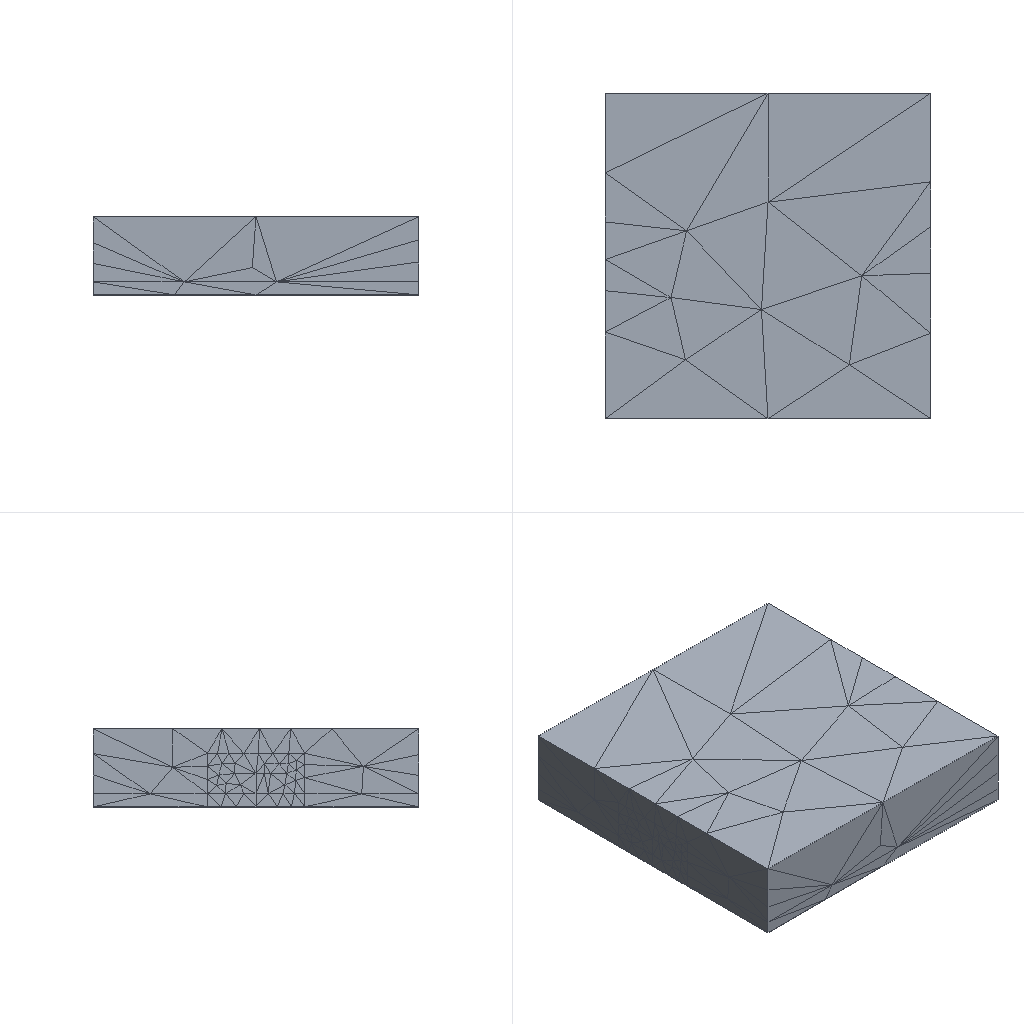Simulation study | ansys electronics desktop
Set-up summary:
category,name,step,type,value,unit,region
solver,ansys_electronics_desktop
units,length mm,,stated,model units
analysis,M15,,HFSS Modal Network,design_type=HFSS
setup,Setup1,M15,HfssDriven,frequency=2.5GHz; max_passes=2; max_delta_s=0.08
sweep,Sweep1,Setup1,Interpolating,1GHz..5GHz n=11 step=
mesh,nodes,,,n/a (no mesh stored)
mesh,elements,,,n/a (no mesh stored)
material,vacuum,,permittivity,1
load,P1,M15,wave port,,,objects 132
load,P2,M15,wave port,,,objects 144
bc,PerfE_TWX736,M15,perfect e,,,objects 118
Ansys Electronics Desktop project file, long lists of numbers shortened, first 729 of 3453 lines:
$begin 'AnsoftProject'
	Created='Wed Sep 30 18:16:02 2026'
	Product='ElectronicsDesktop'
	FileOwnedByWorkbench=false
	$begin 'Desktop'
		Version(2026, 1)
		InfrastructureVersion(1, 0)
		$begin 'FactoryHeader'
			$begin 'geometry3deditor'
				KernelVersion(2, 0)
				ProjectContainsGeometry3D='1'
			$end 'geometry3deditor'
		$end 'FactoryHeader'
	$end 'Desktop'
	UsesAdvancedFeatures=false
	PreviewImageDesignId=1
	NextUniqueID=0
	MoveBackwards=false
	$begin 'HFSSEnvironment'
		Version(1, 0)
	$end 'HFSSEnvironment'
	$begin 'PlanarEMEnvironment'
		Version(1, 0)
	$end 'PlanarEMEnvironment'
	$begin 'Q3DEnvironment'
		Version(1, 0)
	$end 'Q3DEnvironment'
	$begin '2DExtractorEnvironment'
		Version(1, 0)
	$end '2DExtractorEnvironment'
	$begin 'NexximEnvironment'
		Version(1, 0)
	$end 'NexximEnvironment'
	$begin 'NexximNetlistEnvironment'
		Version(1, 0)
	$end 'NexximNetlistEnvironment'
	$begin 'EmitEnvironment'
		Version(1, 0)
	$end 'EmitEnvironment'
	$begin 'Maxwell3DEnvironment'
		Version(1, 0)
	$end 'Maxwell3DEnvironment'
	$begin 'Maxwell2DEnvironment'
		Version(1, 0)
	$end 'Maxwell2DEnvironment'
	$begin 'RMxprtEnvironment'
		Version(1, 0)
	$end 'RMxprtEnvironment'
	$begin 'MaxCirEnvironment'
		Version(1, 0)
	$end 'MaxCirEnvironment'
	$begin 'SimplorerEnvironment'
		Version(1, 0)
	$end 'SimplorerEnvironment'
	$begin 'IcepakEnvironment'
		Version(1, 0)
	$end 'IcepakEnvironment'
	$begin 'IcepakFEAEnvironment'
		Version(1, 0)
	$end 'IcepakFEAEnvironment'
	$begin 'SchematicEnvironment'
		Version(1, 0)
	$end 'SchematicEnvironment'
	$begin 'geometry3deditor'
		Version(1, 0)
	$end 'geometry3deditor'
	ReadVersion=12
	$begin 'DesignMgrEnvironment'
		CompInstCounter=1
		GPortCounter=0
		NetCounter=0
		Alias('Ieee;Simplorer Elements\\Ieee', 'Std;Simplorer Elements\\Std', 'Basic_VHDLAMS;Simplorer Elements\\Basic Elements VHDLAMS\\Basic Elements VHDLAMS', 'Digital_Elements;Simplorer Elements\\Digital Elements\\Digital Elements', 'Transformations;Simplorer Elements\\Tools\\Transformations\\Transformations', 'HEV_VHDLAMS;Simplorer Elements\\HEV VHDLAMS\\HEV VHDLAMS', 'automotive_vda;Simplorer Elem
	$end 'DesignMgrEnvironment'
	$begin 'ProjectDatasets'
		NextUniqueID=0
		MoveBackwards=false
		DatasetType='ProjectDatasetType'
		$begin 'DatasetDefinitions'
		$end 'DatasetDefinitions'
	$end 'ProjectDatasets'
	VariableOrders[0:]
	$begin 'Definitions'
		$begin 'Materials'
			$begin 'vacuum'
				CoordinateSystemType='Cartesian'
				BulkOrSurfaceType=1
				$begin 'PhysicsTypes'
					set('Electromagnetic')
				$end 'PhysicsTypes'
				$begin 'AttachedData'
					$begin 'MatAppearanceData'
						property_data='appearance_data'
						Red=230
						Green=230
						Blue=230
						Transparency=0.95
					$end 'MatAppearanceData'
				$end 'AttachedData'
				permittivity='1'
				ModTime=1499970477
				Library='Materials'
				LibLocation='SysLibrary'
				ModSinceLib=false
			$end 'vacuum'
		$end 'Materials'
		$begin 'SurfaceMaterials'
		$end 'SurfaceMaterials'
		$begin 'Scripts'
		$end 'Scripts'
		$begin 'AnsysComponents'
			NextUniqueID=0
			MoveBackwards=false
			$begin 'AnsysComponentDefinitions'
			$end 'AnsysComponentDefinitions'
		$end 'AnsysComponents'
		$begin 'Symbols'
			$begin 'M15'
				ModTime=1790763363
				Library=''
				ModSinceLib=false
				LibLocation='Project'
				HighestLevel=1
				Normalize=true
				InitialLevels(0, 1)
				$begin 'Graphics'
					Rect(0, 0, 0, 0, 0.00254, 0.00254, 0.00508, 0.00508, 0, 0, 0)
					Rect(0, 1, 0, 0, 0.0004233, 0.00254, 0.0004233, 0.0004233, 0, 0, 0)
				$end 'Graphics'
			$end 'M15'
		$end 'Symbols'
		$begin 'DefInfo'
			M15(1002, 0, 0, 0, '', 1790763363, '', 'M15', '', '', '', '', '', 'Design.bmp', '', 'Project', '', '', 1790763363, '', 0, 0)
		$end 'DefInfo'
		$begin 'Compdefs'
			$begin 'M15'
				Library=''
				CircuitEnv=0
				Refbase='U'
				NumParts=1
				ModSinceLib=true
				$begin 'Properties'
					TextProp('Representation', 'SRD', '', 'M15')
					TextProp('Owner', 'SRD', '', 'HFSS')
				$end 'Properties'
				CompExtID=6
				$begin 'Parameters'
					ButtonProp('CosimDefinition', 'D', '', 'Edit', 'Edit', 40501, ButtonPropClientData())
					MenuProp('CoSimulator', 'D', '', 'DefaultNetlist', 0)
				$end 'Parameters'
				$begin 'CosimDefinitions'
					$begin 'CosimDefinition'
						CosimulatorType=4
						CosimDefName='DefaultNetlist'
						IsDefinition=true
						Connect=true
						Data()
						GRef()
					$end 'CosimDefinition'
					DefaultCosim='DefaultNetlist'
				$end 'CosimDefinitions'
			$end 'M15'
		$end 'Compdefs'
	$end 'Definitions'
	DesignIDServer=2
	MoveBackwards=false
	$begin 'HFSSModel'
		RepRewriteV2=true
		Name='M15'
		DesignID=0
		'Use Advanced DC Extrapolation'=false
		'Use Power S'=false
		'Export FRTM After Simulation'=false
		'Export Rays After Simulation'=false
		'Export After Simulation'=false
		'Allow Material Override'=false
		'Calculate Lossy Dielectrics'=false
		'Perform Minimal validation'=false
		$begin 'TemperatureSettings'
			IncludeTemperatureDependence=false
			EnableFeedback=false
			Temperatures(6, '22cel', 34, '22cel', 62, '22cel', 90, '22cel', 118, '22cel', 132, '22cel', 144, '22cel', 156, '22cel')
		$end 'TemperatureSettings'
		ObjsEnabledForDeformation()
		'Port Validation Settings'='Standard'
		'Save Adaptive support files'=false
		SolutionType='HFSS Modal Network'
		$begin 'DrivenOptions'
			AutoOpen=false
		$end 'DrivenOptions'
		HasTransientSetups=false
		MaterialDensity=1
		MassOfTissue=1
		VoxelSize=1
		TissueObjectList=-1
		AverageSarMethod=0
		UseAutoDCThickness=true
		HaveZwaveSupport=true
		SolveInsideThreshold=100000
		RequireBodyFaceInfo=false
		$begin 'OutputVariable'
			NextUniqueID=0
			MoveBackwards=false
		$end 'OutputVariable'
		$begin 'ModelSetup'
			$begin 'DesignDatasets'
				NextUniqueID=0
				MoveBackwards=false
				DatasetType='DesignDatasetType'
				$begin 'DatasetDefinitions'
				$end 'DatasetDefinitions'
			$end 'DesignDatasets'
			VariableOrders[0:]
			$begin 'Editor3D Doc Preferences'
				BackgroundColorVersion=1
				'Plane Background'=0
				'Need Lights'=true
				'Ambient Light'=8355711
				'Num Lights'=1
				Light0[4: 16777215, 0.75, -0.15, -0.63]
				Ver=2
			$end 'Editor3D Doc Preferences'
			SnapMode=31
			WorkingCS=1
			$begin 'GeometryCore'
				BlockVersionID=3
				DataVersion=2
				NativeKernel='PARASOLID'
				NativeKernelVersionID=26
				Units='mm'
				ModelExtents=10000
				InstanceID=-1
				$begin 'ValidationOptions'
					EntityCheckLevel='Strict'
					IgnoreUnclassifiedObjects=false
					SkipIntersectionChecks=false
				$end 'ValidationOptions'
				ContainsGeomLinkUDM=false
				$begin 'GeometryOperations'
					BlockVersionID=2
					$begin 'AnsoftRangedIDServerManager'
						$begin 'AnsoftRangedIDServer'
							IDServerObjectTypeID=0
							IDServerRangeMin=0
							IDServerRangeMax=2146483647
							NextUniqueID=183
							MoveBackwards=false
						$end 'AnsoftRangedIDServer'
						$begin 'AnsoftRangedIDServer'
							IDServerObjectTypeID=1
							IDServerRangeMin=2146483648
							IDServerRangeMax=2146485547
							NextUniqueID=2146483654
							MoveBackwards=false
						$end 'AnsoftRangedIDServer'
					$end 'AnsoftRangedIDServerManager'
					StartBackGroundFaceID=2146483648
					$begin 'CoordinateSystems'
					$end 'CoordinateSystems'
					$begin 'OperandCSs'
					$end 'OperandCSs'
					$begin 'SubModelDefinitions'
					$end 'SubModelDefinitions'
					$begin 'Groups'
					$end 'Groups'
					$begin 'UserDefinedModels'
					$end 'UserDefinedModels'
					$begin 'OperandUserDefinedModels'
					$end 'OperandUserDefinedModels'
					$begin 'ToplevelParts'
						$begin 'GeometryPart'
							$begin 'Attributes'
								Name='Sub'
								Flags=''
								Color='(230 230 230)'
								Transparency=0.8
								PartCoordinateSystem=1
								UDMId=-1
								GroupId=-1
								MaterialValue='"vacuum"'
								SurfaceMaterialValue='""'
								SolveInside=true
								ShellElement=false
								ShellElementThickness='0mm'
								ReferenceTemperature='20cel'
								IsMaterialEditable=true
								IsSurfaceMaterialEditable=true
								UseMaterialAppearance=false
								IsLightweight=false
								IsAlwaysHidden=false
							$end 'Attributes'
							$begin 'PhysicsAttributes'
								SuppressedForPhysics='False'
								SuppressedForPhysicsEditable=true
							$end 'PhysicsAttributes'
							$begin 'Operations'
								$begin 'Operation'
									OperationType='Box'
									ID=5
									ReferenceCoordSystemID=1
									$begin 'BoxParameters'
										KernelVersion=23
										XPosition='-20mm'
										YPosition='-20mm'
										ZPosition='-1.6mm'
										XSize='40mm'
										YSize='40mm'
										ZSize='1.6mm'
									$end 'BoxParameters'
									ParentPartID=6
									ReferenceUDMID=-1
									IsSuppressed=false
									$begin 'OperationIdentity'
										$begin 'Topology'
											NumLumps=1
											NumShells=1
											NumFaces=6
											NumWires=0
											NumLoops=6
											NumCoedges=24
											NumEdges=12
											NumVertices=8
										$end 'Topology'
										BodyID=6
										StartFaceID=7
										StartEdgeID=13
										StartVertexID=25
										NumNewFaces=6
										NumNewEdges=12
										NumNewVertices=8
										FaceNameAndIDMap()
										EdgeNameAndIDMap()
										VertexNameAndIDMap()
									$end 'OperationIdentity'
								$end 'Operation'
							$end 'Operations'
							$begin 'SubregionDependencyInformation'
								ChildSubregions[0:]
							$end 'SubregionDependencyInformation'
						$end 'GeometryPart'
						$begin 'GeometryPart'
							$begin 'Attributes'
								Name='GND'
								Flags=''
								Color='(230 230 230)'
								Transparency=0.8
								PartCoordinateSystem=1
								UDMId=-1
								GroupId=-1
								MaterialValue='"vacuum"'
								SurfaceMaterialValue='""'
								SolveInside=true
								ShellElement=false
								ShellElementThickness='0mm'
								ReferenceTemperature='20cel'
								IsMaterialEditable=true
								IsSurfaceMaterialEditable=true
								UseMaterialAppearance=false
								IsLightweight=false
								IsAlwaysHidden=false
							$end 'Attributes'
							$begin 'PhysicsAttributes'
								SuppressedForPhysics='False'
								SuppressedForPhysicsEditable=true
							$end 'PhysicsAttributes'
							$begin 'Operations'
								$begin 'Operation'
									OperationType='Box'
									ID=33
									ReferenceCoordSystemID=1
									$begin 'BoxParameters'
										KernelVersion=23
										XPosition='-20mm'
										YPosition='-20mm'
										ZPosition='-1.635mm'
										XSize='40mm'
										YSize='40mm'
										ZSize='0.035mm'
									$end 'BoxParameters'
									ParentPartID=34
									ReferenceUDMID=-1
									IsSuppressed=false
									$begin 'OperationIdentity'
										$begin 'Topology'
											NumLumps=1
											NumShells=1
											NumFaces=6
											NumWires=0
											NumLoops=6
											NumCoedges=24
											NumEdges=12
											NumVertices=8
										$end 'Topology'
										BodyID=34
										StartFaceID=35
										StartEdgeID=41
										StartVertexID=53
										NumNewFaces=6
										NumNewEdges=12
										NumNewVertices=8
										FaceNameAndIDMap()
										EdgeNameAndIDMap()
										VertexNameAndIDMap()
									$end 'OperationIdentity'
								$end 'Operation'
							$end 'Operations'
							$begin 'SubregionDependencyInformation'
								ChildSubregions[0:]
							$end 'SubregionDependencyInformation'
						$end 'GeometryPart'
						$begin 'GeometryPart'
							$begin 'Attributes'
								Name='F1'
								Flags=''
								Color='(230 230 230)'
								Transparency=0.8
								PartCoordinateSystem=1
								UDMId=-1
								GroupId=-1
								MaterialValue='"vacuum"'
								SurfaceMaterialValue='""'
								SolveInside=true
								ShellElement=false
								ShellElementThickness='0mm'
								ReferenceTemperature='20cel'
								IsMaterialEditable=true
								IsSurfaceMaterialEditable=true
								UseMaterialAppearance=false
								IsLightweight=false
								IsAlwaysHidden=false
							$end 'Attributes'
							$begin 'PhysicsAttributes'
								SuppressedForPhysics='False'
								SuppressedForPhysicsEditable=true
							$end 'PhysicsAttributes'
							$begin 'Operations'
								$begin 'Operation'
									OperationType='Box'
									ID=61
									ReferenceCoordSystemID=1
									$begin 'BoxParameters'
										KernelVersion=23
										XPosition='-20mm'
										YPosition='-1.5mm'
										ZPosition='0mm'
										XSize='12mm'
										YSize='3mm'
										ZSize='0.035mm'
									$end 'BoxParameters'
									ParentPartID=62
									ReferenceUDMID=-1
									IsSuppressed=false
									$begin 'OperationIdentity'
										$begin 'Topology'
											NumLumps=1
											NumShells=1
											NumFaces=6
											NumWires=0
											NumLoops=6
											NumCoedges=24
											NumEdges=12
											NumVertices=8
										$end 'Topology'
										BodyID=62
										StartFaceID=63
										StartEdgeID=69
										StartVertexID=81
										NumNewFaces=6
										NumNewEdges=12
										NumNewVertices=8
										FaceNameAndIDMap()
										EdgeNameAndIDMap()
										VertexNameAndIDMap()
									$end 'OperationIdentity'
								$end 'Operation'
							$end 'Operations'
							$begin 'SubregionDependencyInformation'
								ChildSubregions[0:]
							$end 'SubregionDependencyInformation'
						$end 'GeometryPart'
						$begin 'GeometryPart'
							$begin 'Attributes'
								Name='F2'
								Flags=''
								Color='(230 230 230)'
								Transparency=0.8
								PartCoordinateSystem=1
								UDMId=-1
								GroupId=-1
								MaterialValue='"vacuum"'
								SurfaceMaterialValue='""'
								SolveInside=true
								ShellElement=false
								ShellElementThickness='0mm'
								ReferenceTemperature='20cel'
								IsMaterialEditable=true
								IsSurfaceMaterialEditable=true
								UseMaterialAppearance=false
								IsLightweight=false
								IsAlwaysHidden=false
							$end 'Attributes'
							$begin 'PhysicsAttributes'
								SuppressedForPhysics='False'
								SuppressedForPhysicsEditable=true
							$end 'PhysicsAttributes'
							$begin 'Operations'
								$begin 'Operation'
									OperationType='Box'
									ID=89
									ReferenceCoordSystemID=1
									$begin 'BoxParameters'
										KernelVersion=23
										XPosition='8mm'
										YPosition='-1.5mm'
										ZPosition='0mm'
										XSize='12mm'
										YSize='3mm'
										ZSize='0.035mm'
									$end 'BoxParameters'
									ParentPartID=90
									ReferenceUDMID=-1
									IsSuppressed=false
									$begin 'OperationIdentity'
										$begin 'Topology'
											NumLumps=1
											NumShells=1
											NumFaces=6
											NumWires=0
											NumLoops=6
											NumCoedges=24
											NumEdges=12
											NumVertices=8
										$end 'Topology'
										BodyID=90
										StartFaceID=91
										StartEdgeID=97
										StartVertexID=109
										NumNewFaces=6
										NumNewEdges=12
										NumNewVertices=8
										FaceNameAndIDMap()
										EdgeNameAndIDMap()
										VertexNameAndIDMap()
									$end 'OperationIdentity'
								$end 'Operation'
							$end 'Operations'
							$begin 'SubregionDependencyInformation'
								ChildSubregions[0:]
							$end 'SubregionDependencyInformation'
						$end 'GeometryPart'
						$begin 'GeometryPart'
							$begin 'Attributes'
								Name='RingO'
								Flags=''
								Color='(230 230 230)'
								Transparency=0.8
								PartCoordinateSystem=1
								UDMId=-1
								GroupId=-1
								MaterialValue='"vacuum"'
								SurfaceMaterialValue='""'
								SolveInside=true
								ShellElement=false
								ShellElementThickness='0mm'
								ReferenceTemperature='20cel'
								IsMaterialEditable=true
								IsSurfaceMaterialEditable=true
								UseMaterialAppearance=false
								IsLightweight=false
								IsAlwaysHidden=false
							$end 'Attributes'
							$begin 'PhysicsAttributes'
								SuppressedForPhysics='False'
								SuppressedForPhysicsEditable=true
							$end 'PhysicsAttributes'
							$begin 'Operations'
								$begin 'Operation'
									OperationType='Circle'
									ID=117
									ReferenceCoordSystemID=1
									$begin 'CircleParameters'
										KernelVersion=23
										XCenter='0mm'
										YCenter='0mm'
										ZCenter='0mm'
										Radius='10mm'
										WhichAxis='Z'
										NumSegments='0'
									$end 'CircleParameters'
									ParentPartID=118
									ReferenceUDMID=-1
									IsSuppressed=false
									$begin 'OperationIdentity'
										$begin 'Topology'
											NumLumps=1
											NumShells=1
											NumFaces=0
											NumWires=1
											NumLoops=0
											NumCoedges=0
											NumEdges=1
											NumVertices=0
										$end 'Topology'
										BodyID=118
										StartFaceID=-1
										StartEdgeID=119
										StartVertexID=-1
										NumNewFaces=0
										NumNewEdges=1
										NumNewVertices=0
										FaceNameAndIDMap()
										EdgeNameAndIDMap()
										VertexNameAndIDMap()
									$end 'OperationIdentity'
								$end 'Operation'
								$begin 'Operation'
									OperationType='CoverLines'
									ID=121
									$begin 'LocalOperationParameters'
										KernelVersion=23
										LocalOpPart=118
									$end 'LocalOperationParameters'
									ParentPartID=118
									ReferenceUDMID=-1
									IsSuppressed=false
									$begin 'OperationIdentity'
										$begin 'Topology'
											NumLumps=1
											NumShells=1
											NumFaces=1
											NumWires=0
											NumLoops=1
											NumCoedges=1
											NumEdges=1
											NumVertices=0
										$end 'Topology'
										BodyID=-1
										StartFaceID=122
										StartEdgeID=-1
										StartVertexID=-1
										NumNewFaces=1
										NumNewEdges=0
										NumNewVertices=0
										FaceNameAndIDMap()
										EdgeNameAndIDMap()
										VertexNameAndIDMap()
										$begin 'GeomTopolBasedOperationIdentityHelper'
											$begin 'NewFaces'
												$begin 'Face'
													NormalizedSerialNum=0
													ID=122
													$begin 'FaceGeomTopol'
														FaceTopol(1, 1, 1, 0)
														$begin 'FaceGeometry'
															Area=314.159
															FcUVMid(0, 0, 0)
															$begin 'FcTolVts'
															$end 'FcTolVts'
														$end 'FaceGeometry'
													$end 'FaceGeomTopol'
												$end 'Face'
											$end 'NewFaces'
											$begin 'NewEdges'
											$end 'NewEdges'
											$begin 'NewVertices'
											$end 'NewVertices'
										$end 'GeomTopolBasedOperationIdentityHelper'
									$end 'OperationIdentity'
									ParentOperationID=117
								$end 'Operation'
								$begin 'Operation'
									OperationType='Substract'
									ID=129
									$begin 'SubtractParameters'
										KernelVersion=23
										KeepOriginals=false
										TurnOnNBodyBoolean=false
										BlankPart=118
										NumToolParts=1
										ToolParts(124)
									$end 'SubtractParameters'
									ParentPartID=118
									ReferenceUDMID=-1
									IsSuppressed=false
									$begin 'OperationIdentity'
										$begin 'Topology'
											NumLumps=1
											NumShells=1
											NumFaces=1
											NumWires=0
											NumLoops=2
											NumCoedges=2
											NumEdges=2
											NumVertices=0
										$end 'Topology'
										BodyID=-1
										StartFaceID=-1
										StartEdgeID=130
										StartVertexID=-1
										NumNewFaces=0
										NumNewEdges=1
										NumNewVertices=0
										FaceNameAndIDMap()
										EdgeNameAndIDMap()
										VertexNameAndIDMap()
										$begin 'GeomTopolBasedOperationIdentityHelper'
											$begin 'NewFaces'
											$end 'NewFaces'
											$begin 'NewEdges'
												$begin 'Edge'
													NormalizedSerialNum=0
													ID=130
													EdgeFaces(122)
													$begin 'EdTolVts'
													$end 'EdTolVts'
													EdgeMidPoint(-8, 9.79717439317883e-16, 0)
												$end 'Edge'
											$end 'NewEdges'
											$begin 'NewVertices'
											$end 'NewVertices'
										$end 'GeomTopolBasedOperationIdentityHelper'
										$begin 'MergedFaces'
										$end 'MergedFaces'
										$begin 'MergedEdges'
										$end 'MergedEdges'
									$end 'OperationIdentity'
									BlankOperation=121
									NumToolOperations=1
									ToolOperations(127)
								$end 'Operation'
Last 1318 lines:
														$end 'LegendTableAttrib'
														LegendName=''
														ShowTraceName=true
														ShowSolutionName=true
														ShowVariationKey=true
														FileNameDisplayModeInVariationKey=0
														DockMode='None'
													$end 'LegendRenderAttribute'
												$end 'SubMapItem'
											$end 'MainMapItem'
											$begin 'MainMapItem'
												$begin 'SubMapItem'
													DataSourceID=1
													$begin 'LineAxisRenderAttribute'
														DecimalFieldWidth=3
														DecimalFieldPrecision=2
														ManualTitle=''
														ColorVersion=1
														MinScale=0
														MaxScale=1
														TickSpacing=1
														ManualUnits=false
														Units='mm'
														AxisScale='Linear'
														NumberFormat='Auto'
														$begin 'TextFont'
															$begin 'FontAttribute'
																$begin 'Font'
																	HeightInPts=9
																	Width=0
																	Escapement=0
																	Orientation=0
																	Weight=400
																	Italic=0
																	Underline=0
																	StrikeOut=0
																	CharSet=0
																	OutPrecision=7
																	ClipPrecision=48
																	Quality=6
																	PitchAndFamily=0
																	FaceName='Arial'
																$end 'Font'
																ColorVersion=1
															$end 'FontAttribute'
														$end 'TextFont'
														InfMapMode=false
														InfMapValue=1.79769313486232e+306
														AutoRangeMin=true
														AutoRangeMax=true
														AutoSpacing=true
														kNumMinorDivisions=5
														ShowAxisTitle=true
														ShowAxisUnits=true
														vwm='FullWnd'
														viewWndWd=#nan
														ActivateMargins=true
														MarginPercent=0
														NeverCollapse=false
														AxisStripes=true
													$end 'LineAxisRenderAttribute'
												$end 'SubMapItem'
												$begin 'SubMapItem'
													DataSourceID=2
													$begin 'LineAxisRenderAttribute'
														DecimalFieldWidth=3
														DecimalFieldPrecision=2
														ManualTitle=''
														ColorVersion=1
														MinScale=0
														MaxScale=1
														TickSpacing=1
														ManualUnits=false
														Units='mm'
														AxisScale='Linear'
														NumberFormat='Auto'
														$begin 'TextFont'
															$begin 'FontAttribute'
																$begin 'Font'
																	HeightInPts=9
																	Width=0
																	Escapement=0
																	Orientation=0
																	Weight=400
																	Italic=0
																	Underline=0
																	StrikeOut=0
																	CharSet=0
																	OutPrecision=7
																	ClipPrecision=48
																	Quality=6
																	PitchAndFamily=0
																	FaceName='Arial'
																$end 'Font'
																ColorVersion=1
															$end 'FontAttribute'
														$end 'TextFont'
														InfMapMode=false
														InfMapValue=1.79769313486232e+306
														AutoRangeMin=true
														AutoRangeMax=true
														AutoSpacing=true
														kNumMinorDivisions=5
														ShowAxisTitle=true
														ShowAxisUnits=true
														vwm='FullWnd'
														viewWndWd=#nan
														ActivateMargins=true
														MarginPercent=0
														NeverCollapse=false
														AxisStripes=true
													$end 'LineAxisRenderAttribute'
												$end 'SubMapItem'
												$begin 'SubMapItem'
													DataSourceID=8
													$begin 'LineAxisRenderAttribute'
														DecimalFieldWidth=3
														DecimalFieldPrecision=2
														ManualTitle=''
														ColorVersion=1
														MinScale=0
														MaxScale=1
														TickSpacing=1
														ManualUnits=false
														Units='mm'
														AxisScale='Linear'
														NumberFormat='Auto'
														$begin 'TextFont'
															$begin 'FontAttribute'
																$begin 'Font'
																	HeightInPts=9
																	Width=0
																	Escapement=0
																	Orientation=0
																	Weight=400
																	Italic=0
																	Underline=0
																	StrikeOut=0
																	CharSet=0
																	OutPrecision=7
																	ClipPrecision=48
																	Quality=6
																	PitchAndFamily=0
																	FaceName='Arial'
																$end 'Font'
																ColorVersion=1
															$end 'FontAttribute'
														$end 'TextFont'
														InfMapMode=false
														InfMapValue=1.79769313486232e+306
														AutoRangeMin=true
														AutoRangeMax=true
														AutoSpacing=true
														kNumMinorDivisions=5
														ShowAxisTitle=true
														ShowAxisUnits=true
														vwm='FullWnd'
														viewWndWd=#nan
														ActivateMargins=true
														MarginPercent=0
														NeverCollapse=false
														AxisStripes=true
													$end 'LineAxisRenderAttribute'
												$end 'SubMapItem'
												$begin 'SubMapItem'
													DataSourceID=9
													$begin 'LineAxisRenderAttribute'
														DecimalFieldWidth=3
														DecimalFieldPrecision=2
														ManualTitle=''
														ColorVersion=1
														MinScale=0
														MaxScale=1
														TickSpacing=1
														ManualUnits=false
														Units='mm'
														AxisScale='Linear'
														NumberFormat='Auto'
														$begin 'TextFont'
															$begin 'FontAttribute'
																$begin 'Font'
																	HeightInPts=9
																	Width=0
																	Escapement=0
																	Orientation=0
																	Weight=400
																	Italic=0
																	Underline=0
																	StrikeOut=0
																	CharSet=0
																	OutPrecision=7
																	ClipPrecision=48
																	Quality=6
																	PitchAndFamily=0
																	FaceName='Arial'
																$end 'Font'
																ColorVersion=1
															$end 'FontAttribute'
														$end 'TextFont'
														InfMapMode=false
														InfMapValue=1.79769313486232e+306
														AutoRangeMin=true
														AutoRangeMax=true
														AutoSpacing=true
														kNumMinorDivisions=5
														ShowAxisTitle=true
														ShowAxisUnits=true
														vwm='FullWnd'
														viewWndWd=#nan
														ActivateMargins=true
														MarginPercent=0
														NeverCollapse=false
														AxisStripes=true
													$end 'LineAxisRenderAttribute'
												$end 'SubMapItem'
												$begin 'SubMapItem'
													DataSourceID=10
													$begin 'LineAxisRenderAttribute'
														DecimalFieldWidth=3
														DecimalFieldPrecision=2
														ManualTitle=''
														ColorVersion=1
														MinScale=0
														MaxScale=1
														TickSpacing=1
														ManualUnits=false
														Units='mm'
														AxisScale='Linear'
														NumberFormat='Auto'
														$begin 'TextFont'
															$begin 'FontAttribute'
																$begin 'Font'
																	HeightInPts=9
																	Width=0
																	Escapement=0
																	Orientation=0
																	Weight=400
																	Italic=0
																	Underline=0
																	StrikeOut=0
																	CharSet=0
																	OutPrecision=7
																	ClipPrecision=48
																	Quality=6
																	PitchAndFamily=0
																	FaceName='Arial'
																$end 'Font'
																ColorVersion=1
															$end 'FontAttribute'
														$end 'TextFont'
														InfMapMode=false
														InfMapValue=1.79769313486232e+306
														AutoRangeMin=true
														AutoRangeMax=true
														AutoSpacing=true
														kNumMinorDivisions=5
														ShowAxisTitle=true
														ShowAxisUnits=true
														vwm='FullWnd'
														viewWndWd=#nan
														ActivateMargins=true
														MarginPercent=0
														NeverCollapse=false
														AxisStripes=true
													$end 'LineAxisRenderAttribute'
												$end 'SubMapItem'
												$begin 'SubMapItem'
													DataSourceID=11
													$begin 'LineAxisRenderAttribute'
														DecimalFieldWidth=3
														DecimalFieldPrecision=2
														ManualTitle=''
														ColorVersion=1
														MinScale=0
														MaxScale=1
														TickSpacing=1
														ManualUnits=false
														Units='mm'
														AxisScale='Linear'
														NumberFormat='Auto'
														$begin 'TextFont'
															$begin 'FontAttribute'
																$begin 'Font'
																	HeightInPts=9
																	Width=0
																	Escapement=0
																	Orientation=0
																	Weight=400
																	Italic=0
																	Underline=0
																	StrikeOut=0
																	CharSet=0
																	OutPrecision=7
																	ClipPrecision=48
																	Quality=6
																	PitchAndFamily=0
																	FaceName='Arial'
																$end 'Font'
																ColorVersion=1
															$end 'FontAttribute'
														$end 'TextFont'
														InfMapMode=false
														InfMapValue=1.79769313486232e+306
														AutoRangeMin=true
														AutoRangeMax=true
														AutoSpacing=true
														kNumMinorDivisions=5
														ShowAxisTitle=true
														ShowAxisUnits=true
														vwm='FullWnd'
														viewWndWd=#nan
														ActivateMargins=true
														MarginPercent=0
														NeverCollapse=false
														AxisStripes=true
													$end 'LineAxisRenderAttribute'
												$end 'SubMapItem'
												$begin 'SubMapItem'
													DataSourceID=12
													$begin 'LineAxisRenderAttribute'
														DecimalFieldWidth=3
														DecimalFieldPrecision=2
														ManualTitle=''
														ColorVersion=1
														MinScale=0
														MaxScale=1
														TickSpacing=1
														ManualUnits=false
														Units='mm'
														AxisScale='Linear'
														NumberFormat='Auto'
														$begin 'TextFont'
															$begin 'FontAttribute'
																$begin 'Font'
																	HeightInPts=9
																	Width=0
																	Escapement=0
																	Orientation=0
																	Weight=400
																	Italic=0
																	Underline=0
																	StrikeOut=0
																	CharSet=0
																	OutPrecision=7
																	ClipPrecision=48
																	Quality=6
																	PitchAndFamily=0
																	FaceName='Arial'
																$end 'Font'
																ColorVersion=1
															$end 'FontAttribute'
														$end 'TextFont'
														InfMapMode=false
														InfMapValue=1.79769313486232e+306
														AutoRangeMin=true
														AutoRangeMax=true
														AutoSpacing=true
														kNumMinorDivisions=5
														ShowAxisTitle=true
														ShowAxisUnits=true
														vwm='FullWnd'
														viewWndWd=#nan
														ActivateMargins=true
														MarginPercent=0
														NeverCollapse=false
														AxisStripes=true
													$end 'LineAxisRenderAttribute'
												$end 'SubMapItem'
												$begin 'SubMapItem'
													DataSourceID=13
													$begin 'LineAxisRenderAttribute'
														DecimalFieldWidth=3
														DecimalFieldPrecision=2
														ManualTitle=''
														ColorVersion=1
														MinScale=0
														MaxScale=1
														TickSpacing=1
														ManualUnits=false
														Units='mm'
														AxisScale='Linear'
														NumberFormat='Auto'
														$begin 'TextFont'
															$begin 'FontAttribute'
																$begin 'Font'
																	HeightInPts=9
																	Width=0
																	Escapement=0
																	Orientation=0
																	Weight=400
																	Italic=0
																	Underline=0
																	StrikeOut=0
																	CharSet=0
																	OutPrecision=7
																	ClipPrecision=48
																	Quality=6
																	PitchAndFamily=0
																	FaceName='Arial'
																$end 'Font'
																ColorVersion=1
															$end 'FontAttribute'
														$end 'TextFont'
														InfMapMode=false
														InfMapValue=1.79769313486232e+306
														AutoRangeMin=true
														AutoRangeMax=true
														AutoSpacing=true
														kNumMinorDivisions=5
														ShowAxisTitle=true
														ShowAxisUnits=true
														vwm='FullWnd'
														viewWndWd=#nan
														ActivateMargins=true
														MarginPercent=0
														NeverCollapse=false
														AxisStripes=true
													$end 'LineAxisRenderAttribute'
												$end 'SubMapItem'
												$begin 'SubMapItem'
													DataSourceID=14
													$begin 'LineAxisRenderAttribute'
														DecimalFieldWidth=3
														DecimalFieldPrecision=2
														ManualTitle=''
														ColorVersion=1
														MinScale=0
														MaxScale=1
														TickSpacing=1
														ManualUnits=false
														Units='mm'
														AxisScale='Linear'
														NumberFormat='Auto'
														$begin 'TextFont'
															$begin 'FontAttribute'
																$begin 'Font'
																	HeightInPts=9
																	Width=0
																	Escapement=0
																	Orientation=0
																	Weight=400
																	Italic=0
																	Underline=0
																	StrikeOut=0
																	CharSet=0
																	OutPrecision=7
																	ClipPrecision=48
																	Quality=6
																	PitchAndFamily=0
																	FaceName='Arial'
																$end 'Font'
																ColorVersion=1
															$end 'FontAttribute'
														$end 'TextFont'
														InfMapMode=false
														InfMapValue=1.79769313486232e+306
														AutoRangeMin=true
														AutoRangeMax=true
														AutoSpacing=true
														kNumMinorDivisions=5
														ShowAxisTitle=true
														ShowAxisUnits=true
														vwm='FullWnd'
														viewWndWd=#nan
														ActivateMargins=true
														MarginPercent=0
														NeverCollapse=false
														AxisStripes=true
													$end 'LineAxisRenderAttribute'
												$end 'SubMapItem'
												$begin 'SubMapItem'
													DataSourceID=15
													$begin 'LineAxisRenderAttribute'
														DecimalFieldWidth=3
														DecimalFieldPrecision=2
														ManualTitle=''
														ColorVersion=1
														MinScale=0
														MaxScale=1
														TickSpacing=1
														ManualUnits=false
														Units='mm'
														AxisScale='Linear'
														NumberFormat='Auto'
														$begin 'TextFont'
															$begin 'FontAttribute'
																$begin 'Font'
																	HeightInPts=9
																	Width=0
																	Escapement=0
																	Orientation=0
																	Weight=400
																	Italic=0
																	Underline=0
																	StrikeOut=0
																	CharSet=0
																	OutPrecision=7
																	ClipPrecision=48
																	Quality=6
																	PitchAndFamily=0
																	FaceName='Arial'
																$end 'Font'
																ColorVersion=1
															$end 'FontAttribute'
														$end 'TextFont'
														InfMapMode=false
														InfMapValue=1.79769313486232e+306
														AutoRangeMin=true
														AutoRangeMax=true
														AutoSpacing=true
														kNumMinorDivisions=5
														ShowAxisTitle=true
														ShowAxisUnits=true
														vwm='FullWnd'
														viewWndWd=#nan
														ActivateMargins=true
														MarginPercent=0
														NeverCollapse=false
														AxisStripes=true
													$end 'LineAxisRenderAttribute'
												$end 'SubMapItem'
												$begin 'SubMapItem'
													DataSourceID=16
													$begin 'LineAxisRenderAttribute'
														DecimalFieldWidth=3
														DecimalFieldPrecision=2
														ManualTitle=''
														ColorVersion=1
														MinScale=0
														MaxScale=1
														TickSpacing=1
														ManualUnits=false
														Units='mm'
														AxisScale='Linear'
														NumberFormat='Auto'
														$begin 'TextFont'
															$begin 'FontAttribute'
																$begin 'Font'
																	HeightInPts=9
																	Width=0
																	Escapement=0
																	Orientation=0
																	Weight=400
																	Italic=0
																	Underline=0
																	StrikeOut=0
																	CharSet=0
																	OutPrecision=7
																	ClipPrecision=48
																	Quality=6
																	PitchAndFamily=0
																	FaceName='Arial'
																$end 'Font'
																ColorVersion=1
															$end 'FontAttribute'
														$end 'TextFont'
														InfMapMode=false
														InfMapValue=1.79769313486232e+306
														AutoRangeMin=true
														AutoRangeMax=true
														AutoSpacing=true
														kNumMinorDivisions=5
														ShowAxisTitle=true
														ShowAxisUnits=true
														vwm='FullWnd'
														viewWndWd=#nan
														ActivateMargins=true
														MarginPercent=0
														NeverCollapse=false
														AxisStripes=true
													$end 'LineAxisRenderAttribute'
												$end 'SubMapItem'
												$begin 'SubMapItem'
													DataSourceID=17
													$begin 'LineAxisRenderAttribute'
														DecimalFieldWidth=3
														DecimalFieldPrecision=2
														ManualTitle=''
														ColorVersion=1
														MinScale=0
														MaxScale=1
														TickSpacing=1
														ManualUnits=false
														Units='mm'
														AxisScale='Linear'
														NumberFormat='Auto'
														$begin 'TextFont'
															$begin 'FontAttribute'
																$begin 'Font'
																	HeightInPts=9
																	Width=0
																	Escapement=0
																	Orientation=0
																	Weight=400
																	Italic=0
																	Underline=0
																	StrikeOut=0
																	CharSet=0
																	OutPrecision=7
																	ClipPrecision=48
																	Quality=6
																	PitchAndFamily=0
																	FaceName='Arial'
																$end 'Font'
																ColorVersion=1
															$end 'FontAttribute'
														$end 'TextFont'
														InfMapMode=false
														InfMapValue=1.79769313486232e+306
														AutoRangeMin=true
														AutoRangeMax=true
														AutoSpacing=true
														kNumMinorDivisions=5
														ShowAxisTitle=true
														ShowAxisUnits=true
														vwm='FullWnd'
														viewWndWd=#nan
														ActivateMargins=true
														MarginPercent=0
														NeverCollapse=false
														AxisStripes=true
													$end 'LineAxisRenderAttribute'
												$end 'SubMapItem'
												$begin 'SubMapItem'
													DataSourceID=18
													$begin 'LineAxisRenderAttribute'
														DecimalFieldWidth=3
														DecimalFieldPrecision=2
														ManualTitle=''
														ColorVersion=1
														MinScale=0
														MaxScale=1
														TickSpacing=1
														ManualUnits=false
														Units='mm'
														AxisScale='Linear'
														NumberFormat='Auto'
														$begin 'TextFont'
															$begin 'FontAttribute'
																$begin 'Font'
																	HeightInPts=9
																	Width=0
																	Escapement=0
																	Orientation=0
																	Weight=400
																	Italic=0
																	Underline=0
																	StrikeOut=0
																	CharSet=0
																	OutPrecision=7
																	ClipPrecision=48
																	Quality=6
																	PitchAndFamily=0
																	FaceName='Arial'
																$end 'Font'
																ColorVersion=1
															$end 'FontAttribute'
														$end 'TextFont'
														InfMapMode=false
														InfMapValue=1.79769313486232e+306
														AutoRangeMin=true
														AutoRangeMax=true
														AutoSpacing=true
														kNumMinorDivisions=5
														ShowAxisTitle=true
														ShowAxisUnits=true
														vwm='FullWnd'
														viewWndWd=#nan
														ActivateMargins=true
														MarginPercent=0
														NeverCollapse=false
														AxisStripes=true
													$end 'LineAxisRenderAttribute'
												$end 'SubMapItem'
												$begin 'SubMapItem'
													DataSourceID=19
													$begin 'LineAxisRenderAttribute'
														DecimalFieldWidth=3
														DecimalFieldPrecision=2
														ManualTitle=''
														ColorVersion=1
														MinScale=0
														MaxScale=1
														TickSpacing=1
														ManualUnits=false
														Units='mm'
														AxisScale='Linear'
														NumberFormat='Auto'
														$begin 'TextFont'
															$begin 'FontAttribute'
																$begin 'Font'
																	HeightInPts=9
																	Width=0
																	Escapement=0
																	Orientation=0
																	Weight=400
																	Italic=0
																	Underline=0
																	StrikeOut=0
																	CharSet=0
																	OutPrecision=7
																	ClipPrecision=48
																	Quality=6
																	PitchAndFamily=0
																	FaceName='Arial'
																$end 'Font'
																ColorVersion=1
															$end 'FontAttribute'
														$end 'TextFont'
														InfMapMode=false
														InfMapValue=1.79769313486232e+306
														AutoRangeMin=true
														AutoRangeMax=true
														AutoSpacing=true
														kNumMinorDivisions=5
														ShowAxisTitle=true
														ShowAxisUnits=true
														vwm='FullWnd'
														viewWndWd=#nan
														ActivateMargins=true
														MarginPercent=0
														NeverCollapse=false
														AxisStripes=true
													$end 'LineAxisRenderAttribute'
												$end 'SubMapItem'
												$begin 'SubMapItem'
													DataSourceID=20
													$begin 'LineAxisRenderAttribute'
														DecimalFieldWidth=3
														DecimalFieldPrecision=2
														ManualTitle=''
														ColorVersion=1
														MinScale=0
														MaxScale=1
														TickSpacing=1
														ManualUnits=false
														Units='mm'
														AxisScale='Linear'
														NumberFormat='Auto'
														$begin 'TextFont'
															$begin 'FontAttribute'
																$begin 'Font'
																	HeightInPts=9
																	Width=0
																	Escapement=0
																	Orientation=0
																	Weight=400
																	Italic=0
																	Underline=0
																	StrikeOut=0
																	CharSet=0
																	OutPrecision=7
																	ClipPrecision=48
																	Quality=6
																	PitchAndFamily=0
																	FaceName='Arial'
																$end 'Font'
																ColorVersion=1
															$end 'FontAttribute'
														$end 'TextFont'
														InfMapMode=false
														InfMapValue=1.79769313486232e+306
														AutoRangeMin=true
														AutoRangeMax=true
														AutoSpacing=true
														kNumMinorDivisions=5
														ShowAxisTitle=true
														ShowAxisUnits=true
														vwm='FullWnd'
														viewWndWd=#nan
														ActivateMargins=true
														MarginPercent=0
														NeverCollapse=false
														AxisStripes=true
													$end 'LineAxisRenderAttribute'
												$end 'SubMapItem'
												$begin 'SubMapItem'
													DataSourceID=21
													$begin 'LineAxisRenderAttribute'
														DecimalFieldWidth=3
														DecimalFieldPrecision=2
														ManualTitle=''
														ColorVersion=1
														MinScale=0
														MaxScale=1
														TickSpacing=1
														ManualUnits=false
														Units='mm'
														AxisScale='Linear'
														NumberFormat='Auto'
														$begin 'TextFont'
															$begin 'FontAttribute'
																$begin 'Font'
																	HeightInPts=9
																	Width=0
																	Escapement=0
																	Orientation=0
																	Weight=400
																	Italic=0
																	Underline=0
																	StrikeOut=0
																	CharSet=0
																	OutPrecision=7
																	ClipPrecision=48
																	Quality=6
																	PitchAndFamily=0
																	FaceName='Arial'
																$end 'Font'
																ColorVersion=1
															$end 'FontAttribute'
														$end 'TextFont'
														InfMapMode=false
														InfMapValue=1.79769313486232e+306
														AutoRangeMin=true
														AutoRangeMax=true
														AutoSpacing=true
														kNumMinorDivisions=5
														ShowAxisTitle=true
														ShowAxisUnits=true
														vwm='FullWnd'
														viewWndWd=#nan
														ActivateMargins=true
														MarginPercent=0
														NeverCollapse=false
														AxisStripes=true
													$end 'LineAxisRenderAttribute'
												$end 'SubMapItem'
												$begin 'SubMapItem'
													DataSourceID=22
													$begin 'LineAxisRenderAttribute'
														DecimalFieldWidth=3
														DecimalFieldPrecision=2
														ManualTitle=''
														ColorVersion=1
														MinScale=0
														MaxScale=1
														TickSpacing=1
														ManualUnits=false
														Units='mm'
														AxisScale='Linear'
														NumberFormat='Auto'
														$begin 'TextFont'
															$begin 'FontAttribute'
																$begin 'Font'
																	HeightInPts=9
																	Width=0
																	Escapement=0
																	Orientation=0
																	Weight=400
																	Italic=0
																	Underline=0
																	StrikeOut=0
																	CharSet=0
																	OutPrecision=7
																	ClipPrecision=48
																	Quality=6
																	PitchAndFamily=0
																	FaceName='Arial'
																$end 'Font'
																ColorVersion=1
															$end 'FontAttribute'
														$end 'TextFont'
														InfMapMode=false
														InfMapValue=1.79769313486232e+306
														AutoRangeMin=true
														AutoRangeMax=true
														AutoSpacing=true
														kNumMinorDivisions=5
														ShowAxisTitle=true
														ShowAxisUnits=true
														vwm='FullWnd'
														viewWndWd=#nan
														ActivateMargins=true
														MarginPercent=0
														NeverCollapse=false
														AxisStripes=true
													$end 'LineAxisRenderAttribute'
												$end 'SubMapItem'
												$begin 'SubMapItem'
													DataSourceID=23
													$begin 'LineAxisRenderAttribute'
														DecimalFieldWidth=3
														DecimalFieldPrecision=2
														ManualTitle=''
														ColorVersion=1
														MinScale=0
														MaxScale=1
														TickSpacing=1
														ManualUnits=false
														Units='mm'
														AxisScale='Linear'
														NumberFormat='Auto'
														$begin 'TextFont'
															$begin 'FontAttribute'
																$begin 'Font'
																	HeightInPts=9
																	Width=0
																	Escapement=0
																	Orientation=0
																	Weight=400
																	Italic=0
																	Underline=0
																	StrikeOut=0
																	CharSet=0
																	OutPrecision=7
																	ClipPrecision=48
																	Quality=6
																	PitchAndFamily=0
																	FaceName='Arial'
																$end 'Font'
																ColorVersion=1
															$end 'FontAttribute'
														$end 'TextFont'
														InfMapMode=false
														InfMapValue=1.79769313486232e+306
														AutoRangeMin=true
														AutoRangeMax=true
														AutoSpacing=true
														kNumMinorDivisions=5
														ShowAxisTitle=true
														ShowAxisUnits=true
														vwm='FullWnd'
														viewWndWd=#nan
														ActivateMargins=true
														MarginPercent=0
														NeverCollapse=false
														AxisStripes=true
													$end 'LineAxisRenderAttribute'
												$end 'SubMapItem'
												$begin 'SubMapItem'
													DataSourceID=24
													$begin 'LineAxisRenderAttribute'
														DecimalFieldWidth=3
														DecimalFieldPrecision=2
														ManualTitle=''
														ColorVersion=1
														MinScale=0
														MaxScale=1
														TickSpacing=1
														ManualUnits=false
														Units='mm'
														AxisScale='Linear'
														NumberFormat='Auto'
														$begin 'TextFont'
															$begin 'FontAttribute'
																$begin 'Font'
																	HeightInPts=9
																	Width=0
																	Escapement=0
																	Orientation=0
																	Weight=400
																	Italic=0
																	Underline=0
																	StrikeOut=0
																	CharSet=0
																	OutPrecision=7
																	ClipPrecision=48
																	Quality=6
																	PitchAndFamily=0
																	FaceName='Arial'
																$end 'Font'
																ColorVersion=1
															$end 'FontAttribute'
														$end 'TextFont'
														InfMapMode=false
														InfMapValue=1.79769313486232e+306
														AutoRangeMin=true
														AutoRangeMax=true
														AutoSpacing=true
														kNumMinorDivisions=5
														ShowAxisTitle=true
														ShowAxisUnits=true
														vwm='FullWnd'
														viewWndWd=#nan
														ActivateMargins=true
														MarginPercent=0
														NeverCollapse=false
														AxisStripes=true
													$end 'LineAxisRenderAttribute'
												$end 'SubMapItem'
												$begin 'SubMapItem'
													DataSourceID=25
													$begin 'LineAxisRenderAttribute'
														DecimalFieldWidth=3
														DecimalFieldPrecision=2
														ManualTitle=''
														ColorVersion=1
														MinScale=0
														MaxScale=1
														TickSpacing=1
														ManualUnits=false
														Units='mm'
														AxisScale='Linear'
														NumberFormat='Auto'
														$begin 'TextFont'
															$begin 'FontAttribute'
																$begin 'Font'
																	HeightInPts=9
																	Width=0
																	Escapement=0
																	Orientation=0
																	Weight=400
																	Italic=0
																	Underline=0
																	StrikeOut=0
																	CharSet=0
																	OutPrecision=7
																	ClipPrecision=48
																	Quality=6
																	PitchAndFamily=0
																	FaceName='Arial'
																$end 'Font'
																ColorVersion=1
															$end 'FontAttribute'
														$end 'TextFont'
														InfMapMode=false
														InfMapValue=1.79769313486232e+306
														AutoRangeMin=true
														AutoRangeMax=true
														AutoSpacing=true
														kNumMinorDivisions=5
														ShowAxisTitle=true
														ShowAxisUnits=true
														vwm='FullWnd'
														viewWndWd=#nan
														ActivateMargins=true
														MarginPercent=0
														NeverCollapse=false
														AxisStripes=true
													$end 'LineAxisRenderAttribute'
												$end 'SubMapItem'
												$begin 'SubMapItem'
													DataSourceID=26
													$begin 'LineAxisRenderAttribute'
														DecimalFieldWidth=3
														DecimalFieldPrecision=2
														ManualTitle=''
														ColorVersion=1
														MinScale=0
														MaxScale=1
														TickSpacing=1
														ManualUnits=false
														Units='mm'
														AxisScale='Linear'
														NumberFormat='Auto'
														$begin 'TextFont'
															$begin 'FontAttribute'
																$begin 'Font'
																	HeightInPts=9
																	Width=0
																	Escapement=0
																	Orientation=0
																	Weight=400
																	Italic=0
																	Underline=0
																	StrikeOut=0
																	CharSet=0
																	OutPrecision=7
																	ClipPrecision=48
																	Quality=6
																	PitchAndFamily=0
																	FaceName='Arial'
																$end 'Font'
																ColorVersion=1
															$end 'FontAttribute'
														$end 'TextFont'
														InfMapMode=false
														InfMapValue=1.79769313486232e+306
														AutoRangeMin=true
														AutoRangeMax=true
														AutoSpacing=true
														kNumMinorDivisions=5
														ShowAxisTitle=true
														ShowAxisUnits=true
														vwm='FullWnd'
														viewWndWd=#nan
														ActivateMargins=true
														MarginPercent=0
														NeverCollapse=false
														AxisStripes=true
													$end 'LineAxisRenderAttribute'
												$end 'SubMapItem'
											$end 'MainMapItem'
										$end 'PlotAttributeStoreMap'
									$end 'DisplayTypeAttributes'
									$begin 'DocDefaultAttributes'
										$begin 'PlotAttributeStoreMap'
										$end 'PlotAttributeStoreMap'
									$end 'DocDefaultAttributes'
									$begin 'PerViewPlotAttributeStoreMap'
										$begin 'MapItem'
											ItemID=-1
											$begin 'PlotAttributeStoreMap'
												$begin 'MainMapItem'
													$begin 'SubMapItem'
														DataSourceID=4
														$begin 'BasicLayoutAttribute'
															$begin 'LayoutRect'
																Top=986
																Left=1122
																Bottom=9800
																Right=8948
															$end 'LayoutRect'
														$end 'BasicLayoutAttribute'
													$end 'SubMapItem'
													$begin 'SubMapItem'
														DataSourceID=28
														$begin 'BasicLayoutAttribute'
															$begin 'LayoutRect'
																Top=986
																Left=1122
																Bottom=9800
																Right=8948
															$end 'LayoutRect'
														$end 'BasicLayoutAttribute'
													$end 'SubMapItem'
													$begin 'SubMapItem'
														DataSourceID=35
														$begin 'BasicLayoutAttribute'
															$begin 'LayoutRect'
																Top=75
																Left=75
																Bottom=9925
																Right=875
															$end 'LayoutRect'
														$end 'BasicLayoutAttribute'
													$end 'SubMapItem'
												$end 'MainMapItem'
												$begin 'MainMapItem'
													$begin 'SubMapItem'
														DataSourceID=31
														$begin 'CartesianAxisLayoutAttribute'
															$begin 'AxisRect'
																Top=75
																Left=8948
																Bottom=9925
																Right=9925
															$end 'AxisRect'
															$begin 'GridRect'
																Top=986
																Left=1122
																Bottom=9800
																Right=8948
															$end 'GridRect'
															AxisCollapsed=false
															AxisExpandCollapseByUser=false
														$end 'CartesianAxisLayoutAttribute'
													$end 'SubMapItem'
													$begin 'SubMapItem'
														DataSourceID=32
														$begin 'CartesianAxisLayoutAttribute'
															$begin 'AxisRect'
																Top=75
																Left=1122
																Bottom=986
																Right=8948
															$end 'AxisRect'
															$begin 'GridRect'
																Top=986
																Left=1122
																Bottom=9800
																Right=8948
															$end 'GridRect'
															AxisCollapsed=false
															AxisExpandCollapseByUser=false
														$end 'CartesianAxisLayoutAttribute'
													$end 'SubMapItem'
												$end 'MainMapItem'
												$begin 'MainMapItem'
													$begin 'SubMapItem'
														DataSourceID=4
														$begin 'CartesianCurveGroupLayoutAttribute'
															X_spc=500000000
															X_fwd=2
															X_fpr=1
															Y1_spc=0.025
															Y1_fwd=3
															Y1_fpr=3
														$end 'CartesianCurveGroupLayoutAttribute'
													$end 'SubMapItem'
												$end 'MainMapItem'
												$begin 'MainMapItem'
													$begin 'SubMapItem'
														DataSourceID=6
														$begin 'DockableOverlayLayoutAttribute'
															$begin 'Dock_0'
																$begin 'OverlayLayoutAttribute'
																	$begin 'BoundingRect'
																		Top=4850
																		Left=975
																		Bottom=9850
																		Right=8475
																	$end 'BoundingRect'
																	ModifySize=false
																	ModifyPosition=false
																$end 'OverlayLayoutAttribute'
															$end 'Dock_0'
															$begin 'Dock_1'
																$begin 'OverlayLayoutAttribute'
																	$begin 'BoundingRect'
																		Top=5000
																		Left=0
																		Bottom=10000
																		Right=10000
																	$end 'BoundingRect'
																	ModifySize=false
																	ModifyPosition=false
																$end 'OverlayLayoutAttribute'
															$end 'Dock_1'
															$begin 'Dock_2'
																$begin 'OverlayLayoutAttribute'
																	$begin 'BoundingRect'
																		Top=0
																		Left=0
																		Bottom=5000
																		Right=10000
																	$end 'BoundingRect'
																	ModifySize=false
																	ModifyPosition=false
																$end 'OverlayLayoutAttribute'
															$end 'Dock_2'
														$end 'DockableOverlayLayoutAttribute'
													$end 'SubMapItem'
												$end 'MainMapItem'
											$end 'PlotAttributeStoreMap'
											PlotType=1
										$end 'MapItem'
									$end 'PerViewPlotAttributeStoreMap'
									IsViewAttribServer=false
									ViewID=-1
									$begin 'SourceIDMap'
										IDMapItem(0, 0, -1, 37)
									$end 'SourceIDMap'
									$begin 'TraceCharacteristicsMgr'
									$end 'TraceCharacteristicsMgr'
									$begin 'CartesianXMarkerManager'
										RefMarkerID=-1
										CurrentMarkerID=-1
										$begin 'ReferenceCurves'
										$end 'ReferenceCurves'
									$end 'CartesianXMarkerManager'
									$begin 'CartesianYMarkerManager'
									$end 'CartesianYMarkerManager'
									XAxisStackID=-1
									$begin 'AllTransSrcDwg'
										$begin 'PT'
											ID=1
											TransSrcDwg(-1, 0, 35, 1, 31, 2, 32, 5, 6, 27, 28, 37, 38)
										$end 'PT'
									$end 'AllTransSrcDwg'
									$begin 'AllPtSVID'
										PtID(1, -1, 4)
									$end 'AllPtSVID'
								$end 'PlotDisplayDataManager'
							$end 'Report2D'
						$end 'S_Parameters'
					$end 'Reports'
					$begin 'ReportsWindowInfoList'
						$begin 'S_Parameters'
							ReportID=1
							$begin 'WindowInfoList'
							$end 'WindowInfoList'
						$end 'S_Parameters'
					$end 'ReportsWindowInfoList'
				$end 'ReportSetup'
				$begin 'Properties'
				$end 'Properties'
				$begin 'UserDefinedDocument'
					$begin 'Data'
					$end 'Data'
				$end 'UserDefinedDocument'
			$end 'HfssDesignInstance'
		$end 'Instance'
		$begin 'SODInfo'
			$begin 'M15'
				$begin 'CosimDefinition'
					CosimDefName='DefaultNetlist'
					$begin 'SODInstanceMap'
					$end 'SODInstanceMap'
					SODComponentList()
				$end 'CosimDefinition'
			$end 'M15'
		$end 'SODInfo'
	$end 'DataInstances'
	$begin 'WBSystemIDToDesignInstanceIDMap'
	$end 'WBSystemIDToDesignInstanceIDMap'
	$begin 'WBSysIDSysDetails'
	$end 'WBSysIDSysDetails'
	$begin 'WBConnIDConnDetails'
	$end 'WBConnIDConnDetails'
	$begin 'WBMaterialGuidDetails'
		WBMaterialGuidMap()
	$end 'WBMaterialGuidDetails'
	$begin 'MinervaProjectSettingsBlk'
		MinervaRemoteFilePath=''
		FolderContainerString=''
	$end 'MinervaProjectSettingsBlk'
$end 'AnsoftProject'
$begin 'AllReferencedFilesForProject'
$end 'AllReferencedFilesForProject'
$begin 'ProjectPreview'
	ProductName='ElectronicsDesktop'
	MajorVersion=2026
	MinorVersion=1
	IsEncrypted=false
	Thumbnail64=''
	$begin 'DesignInfo'
		DesignName='M15'
		Notes=''
		Factory='HFSS'
		IsSolved=true
		'Nominal Setups'[1: 'Setup1']
		'Nominal Setup Types'[1: '']
		'Optimetrics Setups'[0:]
		'Optimetrics Experiment Types'[0:]
		Image64=''
	$end 'DesignInfo'
$end 'ProjectPreview'
Results summary, first 70 of 138 lines:
result,designs[0].name,1.step,,M15
result,designs[0].design_type,1.step,,HFSS
result,designs[0].solution_type,1.step,,HFSS Modal Network
result,designs[0].setups[0].name,Setup1,,Setup1
result,designs[0].setups[0].SetupType,Setup1,,HfssDriven
result,designs[0].setups[0].SolveType,Setup1,,Single
result,designs[0].setups[0].Frequency,Setup1,,2.5GHz
result,designs[0].setups[0].MaximumPasses,Setup1,,2
result,designs[0].setups[0].MaxDeltaS,Setup1,,0.08
result,designs[0].setups[0].IsEnabled,Setup1,,true
result,designs[0].setups[0].sweeps[0].name,Sweep1,,Sweep1
result,designs[0].setups[0].sweeps[0].RangeType,Sweep1,,LinearCount
result,designs[0].setups[0].sweeps[0].RangeStart,Sweep1,,1GHz
result,designs[0].setups[0].sweeps[0].RangeEnd,Sweep1,,5GHz
result,designs[0].setups[0].sweeps[0].RangeCount,Sweep1,,11
result,designs[0].setups[0].sweeps[0].Type,Sweep1,,Interpolating
result,designs[0].setups[0].sweeps[0].IsEnabled,Sweep1,,true
result,designs[0].boundaries[0].name,PerfE_TWX736,,PerfE_TWX736
result,designs[0].boundaries[0].BoundType,PerfE_TWX736,,Perfect E
result,designs[0].excitations[0].name,P1,,P1
result,designs[0].excitations[0].BoundType,P1,,Wave Port
result,designs[0].excitations[0].WavePortType,P1,,Modal
result,designs[0].excitations[0].NumModes,P1,,1
result,designs[0].excitations[1].name,P2,,P2
result,designs[0].excitations[1].BoundType,P2,,Wave Port
result,designs[0].excitations[1].WavePortType,P2,,Modal
result,designs[0].excitations[1].NumModes,P2,,1
result,designs[0].materials_assigned[0],1.step,,vacuum
result,designs[0].objects,1.step,,9
result,designs[0].model_units,1.step,,mm
result,designs[0].valid_solutions[0],1.step,,Setup1 : AdaptivePass
result,designs[0].valid_solutions[1],1.step,,Setup1 : LastAdaptive
result,designs[0].valid_solutions[2],1.step,,Setup1 : Sweep1
result,designs[0].sparams[0].freq_hz[1],1.step,,1e+09
result,designs[0].sparams[0].freq_hz[2],1.step,,1.4e+09
result,designs[0].sparams[0].freq_hz[3],1.step,,1.8e+09
result,designs[0].sparams[0].freq_hz[4],1.step,,2.2e+09
result,designs[0].sparams[0].freq_hz[5],1.step,,2.6e+09
result,designs[0].sparams[0].freq_hz[6],1.step,,3e+09
result,designs[0].sparams[0].freq_hz[7],1.step,,3.4e+09
result,designs[0].sparams[0].freq_hz[8],1.step,,3.8e+09
result,designs[0].sparams[0].freq_hz[9],1.step,,4.2e+09
result,designs[0].sparams[0].freq_hz[10],1.step,,4.6e+09
result,designs[0].sparams[0].freq_hz[11],1.step,,5e+09
result,designs[0].sparams[0].expr,1.step,,"dB(S(P1,P1))"
result,designs[0].sparams[0].min_db,1.step,,-0.2133
result,designs[0].sparams[0].solution,1.step,,Setup1 : Sweep1
result,designs[0].sparams[0].value_db[1],1.step,,-0.0005399
result,designs[0].sparams[0].value_db[2],1.step,,-0.0008122
result,designs[0].sparams[0].value_db[3],1.step,,-0.001057
result,designs[0].sparams[0].value_db[4],1.step,,-0.00132
result,designs[0].sparams[0].value_db[5],1.step,,-0.001679
result,designs[0].sparams[0].value_db[6],1.step,,-0.002258
result,designs[0].sparams[0].value_db[7],1.step,,-0.003317
result,designs[0].sparams[0].value_db[8],1.step,,-0.005535
result,designs[0].sparams[0].value_db[9],1.step,,-0.01119
result,designs[0].sparams[0].value_db[10],1.step,,-0.03172
result,designs[0].sparams[0].value_db[11],1.step,,-0.2133
result,designs[0].sparams[0].max_db,1.step,,-0.0005399
result,designs[0].sparams[1].freq_hz[1],1.step,,1e+09
result,designs[0].sparams[1].freq_hz[2],1.step,,1.4e+09
result,designs[0].sparams[1].freq_hz[3],1.step,,1.8e+09
result,designs[0].sparams[1].freq_hz[4],1.step,,2.2e+09
result,designs[0].sparams[1].freq_hz[5],1.step,,2.6e+09
result,designs[0].sparams[1].freq_hz[6],1.step,,3e+09
result,designs[0].sparams[1].freq_hz[7],1.step,,3.4e+09
result,designs[0].sparams[1].freq_hz[8],1.step,,3.8e+09
result,designs[0].sparams[1].freq_hz[9],1.step,,4.2e+09
result,designs[0].sparams[1].freq_hz[10],1.step,,4.6e+09
result,designs[0].sparams[1].freq_hz[11],1.step,,5e+09